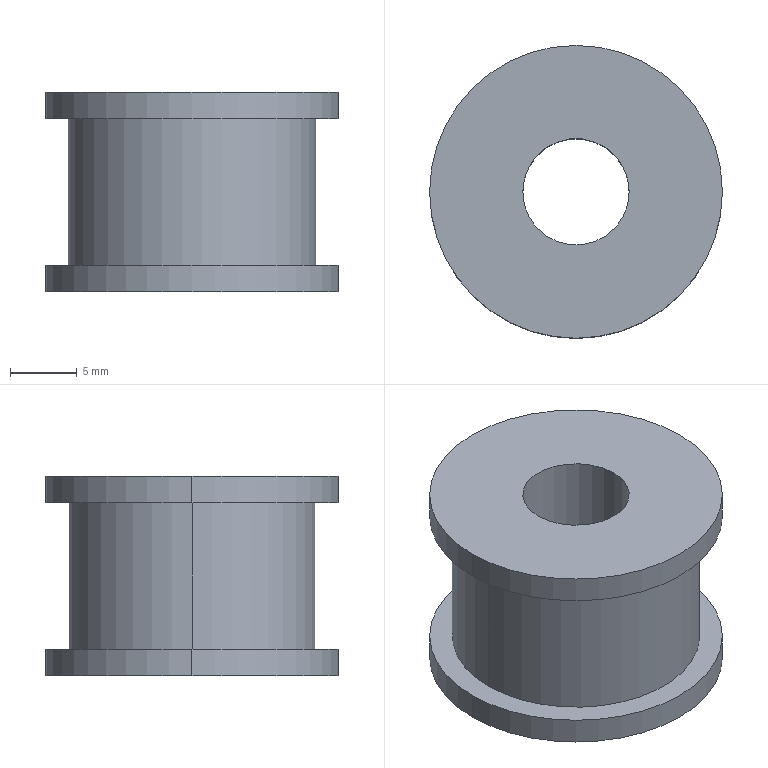Part | SolidWorks | features BaseBody 1 | 1 solid | 12 faces | box 22 x 22 x 15 mm | volume 3752 mm3 | cylinder 8 | plane 4 | commonest cylinder face diameters 22 x4 8 x2 18.59 x2
STEP:
#1=CARTESIAN_POINT('',(-9.295,0.,13.));
#2=VERTEX_POINT('',#1);
#3=CARTESIAN_POINT('',(9.295,0.,13.));
#4=VERTEX_POINT('',#3);
#5=CARTESIAN_POINT('',(0.,0.,13.));
#6=DIRECTION('',(0.,0.,-1.));
#7=DIRECTION('',(-1.,0.,0.));
#8=AXIS2_PLACEMENT_3D('',#5,#6,#7);
#9=CIRCLE('',#8,9.295);
#10=EDGE_CURVE('',#2,#4,#9,.T.);
#11=ORIENTED_EDGE('',*,*,#10,.T.);
#12=CARTESIAN_POINT('',(9.295,0.,2.));
#13=VERTEX_POINT('',#12);
#14=CARTESIAN_POINT('',(9.295,0.,7.5));
#15=DIRECTION('',(0.,0.,-1.));
#16=VECTOR('',#15,1000.);
#17=LINE('',#14,#16);
#18=EDGE_CURVE('',#4,#13,#17,.T.);
#19=ORIENTED_EDGE('',*,*,#18,.T.);
#20=CARTESIAN_POINT('',(-9.295,0.,2.));
#21=VERTEX_POINT('',#20);
#22=CARTESIAN_POINT('',(0.,0.,2.));
#23=DIRECTION('',(0.,0.,1.));
#24=DIRECTION('',(-1.,0.,0.));
#25=AXIS2_PLACEMENT_3D('',#22,#23,#24);
#26=CIRCLE('',#25,9.295);
#27=EDGE_CURVE('',#13,#21,#26,.T.);
#28=ORIENTED_EDGE('',*,*,#27,.T.);
#29=CARTESIAN_POINT('',(-9.295,0.,7.5));
#30=DIRECTION('',(0.,0.,-1.));
#31=VECTOR('',#30,1000.);
#32=LINE('',#29,#31);
#33=EDGE_CURVE('',#2,#21,#32,.T.);
#34=ORIENTED_EDGE('',*,*,#33,.F.);
#35=EDGE_LOOP('',(#11,#19,#28,#34));
#36=FACE_OUTER_BOUND('',#35,.T.);
#37=CARTESIAN_POINT('',(0.,0.,7.5));
#38=DIRECTION('',(0.,0.,-1.));
#39=DIRECTION('',(-1.,0.,0.));
#40=AXIS2_PLACEMENT_3D('',#37,#38,#39);
#41=CYLINDRICAL_SURFACE('',#40,9.295);
#42=ADVANCED_FACE('',(#36),#41,.T.);
#43=CARTESIAN_POINT('',(11.,0.,0.));
#44=VERTEX_POINT('',#43);
#45=CARTESIAN_POINT('',(-11.,0.,0.));
#46=VERTEX_POINT('',#45);
#47=CARTESIAN_POINT('',(0.,0.,0.));
#48=DIRECTION('',(0.,0.,1.));
#49=DIRECTION('',(1.,0.,0.));
#50=AXIS2_PLACEMENT_3D('',#47,#48,#49);
#51=CIRCLE('',#50,11.);
#52=EDGE_CURVE('',#44,#46,#51,.T.);
#53=ORIENTED_EDGE('',*,*,#52,.T.);
#54=CARTESIAN_POINT('',(-11.,0.,2.));
#55=VERTEX_POINT('',#54);
#56=CARTESIAN_POINT('',(-11.,0.,0.));
#57=DIRECTION('',(0.,0.,1.));
#58=VECTOR('',#57,1000.);
#59=LINE('',#56,#58);
#60=EDGE_CURVE('',#46,#55,#59,.T.);
#61=ORIENTED_EDGE('',*,*,#60,.T.);
#62=CARTESIAN_POINT('',(11.,0.,2.));
#63=VERTEX_POINT('',#62);
#64=CARTESIAN_POINT('',(0.,0.,2.));
#65=DIRECTION('',(0.,0.,-1.));
#66=DIRECTION('',(1.,0.,0.));
#67=AXIS2_PLACEMENT_3D('',#64,#65,#66);
#68=CIRCLE('',#67,11.);
#69=EDGE_CURVE('',#55,#63,#68,.T.);
#70=ORIENTED_EDGE('',*,*,#69,.T.);
#71=CARTESIAN_POINT('',(11.,0.,0.));
#72=DIRECTION('',(0.,0.,1.));
#73=VECTOR('',#72,1000.);
#74=LINE('',#71,#73);
#75=EDGE_CURVE('',#44,#63,#74,.T.);
#76=ORIENTED_EDGE('',*,*,#75,.F.);
#77=EDGE_LOOP('',(#53,#61,#70,#76));
#78=FACE_OUTER_BOUND('',#77,.T.);
#79=CARTESIAN_POINT('',(0.,0.,0.));
#80=DIRECTION('',(0.,0.,1.));
#81=DIRECTION('',(1.,0.,0.));
#82=AXIS2_PLACEMENT_3D('',#79,#80,#81);
#83=CYLINDRICAL_SURFACE('',#82,11.);
#84=ADVANCED_FACE('',(#78),#83,.T.);
#85=CARTESIAN_POINT('',(11.,0.,13.));
#86=VERTEX_POINT('',#85);
#87=CARTESIAN_POINT('',(-11.,0.,13.));
#88=VERTEX_POINT('',#87);
#89=CARTESIAN_POINT('',(0.,0.,13.));
#90=DIRECTION('',(0.,0.,1.));
#91=DIRECTION('',(1.,0.,0.));
#92=AXIS2_PLACEMENT_3D('',#89,#90,#91);
#93=CIRCLE('',#92,11.);
#94=EDGE_CURVE('',#86,#88,#93,.T.);
#95=ORIENTED_EDGE('',*,*,#94,.T.);
#96=CARTESIAN_POINT('',(-11.,0.,15.));
#97=VERTEX_POINT('',#96);
#98=CARTESIAN_POINT('',(-11.,0.,0.));
#99=DIRECTION('',(0.,0.,1.));
#100=VECTOR('',#99,1000.);
#101=LINE('',#98,#100);
#102=EDGE_CURVE('',#88,#97,#101,.T.);
#103=ORIENTED_EDGE('',*,*,#102,.T.);
#104=CARTESIAN_POINT('',(11.,0.,15.));
#105=VERTEX_POINT('',#104);
#106=CARTESIAN_POINT('',(0.,0.,15.));
#107=DIRECTION('',(0.,0.,-1.));
#108=DIRECTION('',(1.,0.,0.));
#109=AXIS2_PLACEMENT_3D('',#106,#107,#108);
#110=CIRCLE('',#109,11.);
#111=EDGE_CURVE('',#97,#105,#110,.T.);
#112=ORIENTED_EDGE('',*,*,#111,.T.);
#113=CARTESIAN_POINT('',(11.,0.,0.));
#114=DIRECTION('',(0.,0.,1.));
#115=VECTOR('',#114,1000.);
#116=LINE('',#113,#115);
#117=EDGE_CURVE('',#86,#105,#116,.T.);
#118=ORIENTED_EDGE('',*,*,#117,.F.);
#119=EDGE_LOOP('',(#95,#103,#112,#118));
#120=FACE_OUTER_BOUND('',#119,.T.);
#121=CARTESIAN_POINT('',(0.,0.,0.));
#122=DIRECTION('',(0.,0.,1.));
#123=DIRECTION('',(1.,0.,0.));
#124=AXIS2_PLACEMENT_3D('',#121,#122,#123);
#125=CYLINDRICAL_SURFACE('',#124,11.);
#126=ADVANCED_FACE('',(#120),#125,.T.);
#127=CARTESIAN_POINT('',(-4.,0.,0.));
#128=VERTEX_POINT('',#127);
#129=CARTESIAN_POINT('',(4.,0.,0.));
#130=VERTEX_POINT('',#129);
#131=CARTESIAN_POINT('',(0.,0.,0.));
#132=DIRECTION('',(0.,0.,1.));
#133=DIRECTION('',(1.,0.,0.));
#134=AXIS2_PLACEMENT_3D('',#131,#132,#133);
#135=CIRCLE('',#134,4.);
#136=EDGE_CURVE('',#128,#130,#135,.T.);
#137=ORIENTED_EDGE('',*,*,#136,.F.);
#138=CARTESIAN_POINT('',(-4.,0.,15.));
#139=VERTEX_POINT('',#138);
#140=CARTESIAN_POINT('',(-4.,0.,-19.54));
#141=DIRECTION('',(0.,0.,1.));
#142=VECTOR('',#141,1000.);
#143=LINE('',#140,#142);
#144=EDGE_CURVE('',#128,#139,#143,.T.);
#145=ORIENTED_EDGE('',*,*,#144,.T.);
#146=CARTESIAN_POINT('',(4.,0.,15.));
#147=VERTEX_POINT('',#146);
#148=CARTESIAN_POINT('',(0.,0.,15.));
#149=DIRECTION('',(0.,0.,1.));
#150=DIRECTION('',(1.,0.,0.));
#151=AXIS2_PLACEMENT_3D('',#148,#149,#150);
#152=CIRCLE('',#151,4.);
#153=EDGE_CURVE('',#139,#147,#152,.T.);
#154=ORIENTED_EDGE('',*,*,#153,.T.);
#155=CARTESIAN_POINT('',(4.,0.,-19.54));
#156=DIRECTION('',(0.,0.,1.));
#157=VECTOR('',#156,1000.);
#158=LINE('',#155,#157);
#159=EDGE_CURVE('',#130,#147,#158,.T.);
#160=ORIENTED_EDGE('',*,*,#159,.F.);
#161=EDGE_LOOP('',(#137,#145,#154,#160));
#162=FACE_OUTER_BOUND('',#161,.T.);
#163=CARTESIAN_POINT('',(0.,0.,-19.54));
#164=DIRECTION('',(0.,0.,1.));
#165=DIRECTION('',(1.,0.,0.));
#166=AXIS2_PLACEMENT_3D('',#163,#164,#165);
#167=CYLINDRICAL_SURFACE('',#166,4.);
#168=ADVANCED_FACE('',(#162),#167,.F.);
#169=ORIENTED_EDGE('',*,*,#18,.F.);
#170=CARTESIAN_POINT('',(0.,0.,13.));
#171=DIRECTION('',(0.,0.,-1.));
#172=DIRECTION('',(-1.,0.,0.));
#173=AXIS2_PLACEMENT_3D('',#170,#171,#172);
#174=CIRCLE('',#173,9.295);
#175=EDGE_CURVE('',#4,#2,#174,.T.);
#176=ORIENTED_EDGE('',*,*,#175,.T.);
#177=ORIENTED_EDGE('',*,*,#33,.T.);
#178=CARTESIAN_POINT('',(0.,0.,2.));
#179=DIRECTION('',(0.,0.,1.));
#180=DIRECTION('',(-1.,0.,0.));
#181=AXIS2_PLACEMENT_3D('',#178,#179,#180);
#182=CIRCLE('',#181,9.295);
#183=EDGE_CURVE('',#21,#13,#182,.T.);
#184=ORIENTED_EDGE('',*,*,#183,.T.);
#185=EDGE_LOOP('',(#169,#176,#177,#184));
#186=FACE_OUTER_BOUND('',#185,.T.);
#187=CARTESIAN_POINT('',(0.,0.,7.5));
#188=DIRECTION('',(0.,0.,-1.));
#189=DIRECTION('',(-1.,0.,0.));
#190=AXIS2_PLACEMENT_3D('',#187,#188,#189);
#191=CYLINDRICAL_SURFACE('',#190,9.295);
#192=ADVANCED_FACE('',(#186),#191,.T.);
#193=ORIENTED_EDGE('',*,*,#183,.F.);
#194=ORIENTED_EDGE('',*,*,#27,.F.);
#195=EDGE_LOOP('',(#193,#194));
#196=FACE_BOUND('',#195,.T.);
#197=CARTESIAN_POINT('',(0.,0.,2.));
#198=DIRECTION('',(0.,0.,-1.));
#199=DIRECTION('',(1.,0.,0.));
#200=AXIS2_PLACEMENT_3D('',#197,#198,#199);
#201=CIRCLE('',#200,11.);
#202=EDGE_CURVE('',#63,#55,#201,.T.);
#203=ORIENTED_EDGE('',*,*,#202,.F.);
#204=ORIENTED_EDGE('',*,*,#69,.F.);
#205=EDGE_LOOP('',(#203,#204));
#206=FACE_OUTER_BOUND('',#205,.T.);
#207=CARTESIAN_POINT('',(0.,10.148,2.));
#208=DIRECTION('',(0.,0.,-1.));
#209=DIRECTION('',(-1.,0.,0.));
#210=AXIS2_PLACEMENT_3D('',#207,#208,#209);
#211=PLANE('',#210);
#212=ADVANCED_FACE('',(#196,#206),#211,.F.);
#213=ORIENTED_EDGE('',*,*,#10,.F.);
#214=ORIENTED_EDGE('',*,*,#175,.F.);
#215=EDGE_LOOP('',(#213,#214));
#216=FACE_BOUND('',#215,.T.);
#217=ORIENTED_EDGE('',*,*,#94,.F.);
#218=CARTESIAN_POINT('',(0.,0.,13.));
#219=DIRECTION('',(0.,0.,1.));
#220=DIRECTION('',(1.,0.,0.));
#221=AXIS2_PLACEMENT_3D('',#218,#219,#220);
#222=CIRCLE('',#221,11.);
#223=EDGE_CURVE('',#88,#86,#222,.T.);
#224=ORIENTED_EDGE('',*,*,#223,.F.);
#225=EDGE_LOOP('',(#217,#224));
#226=FACE_OUTER_BOUND('',#225,.T.);
#227=CARTESIAN_POINT('',(0.,10.148,13.));
#228=DIRECTION('',(0.,0.,1.));
#229=DIRECTION('',(1.,0.,0.));
#230=AXIS2_PLACEMENT_3D('',#227,#228,#229);
#231=PLANE('',#230);
#232=ADVANCED_FACE('',(#216,#226),#231,.F.);
#233=ORIENTED_EDGE('',*,*,#60,.F.);
#234=CARTESIAN_POINT('',(0.,0.,0.));
#235=DIRECTION('',(0.,0.,1.));
#236=DIRECTION('',(1.,0.,0.));
#237=AXIS2_PLACEMENT_3D('',#234,#235,#236);
#238=CIRCLE('',#237,11.);
#239=EDGE_CURVE('',#46,#44,#238,.T.);
#240=ORIENTED_EDGE('',*,*,#239,.T.);
#241=ORIENTED_EDGE('',*,*,#75,.T.);
#242=ORIENTED_EDGE('',*,*,#202,.T.);
#243=EDGE_LOOP('',(#233,#240,#241,#242));
#244=FACE_OUTER_BOUND('',#243,.T.);
#245=CARTESIAN_POINT('',(0.,0.,0.));
#246=DIRECTION('',(0.,0.,1.));
#247=DIRECTION('',(1.,0.,0.));
#248=AXIS2_PLACEMENT_3D('',#245,#246,#247);
#249=CYLINDRICAL_SURFACE('',#248,11.);
#250=ADVANCED_FACE('',(#244),#249,.T.);
#251=ORIENTED_EDGE('',*,*,#102,.F.);
#252=ORIENTED_EDGE('',*,*,#223,.T.);
#253=ORIENTED_EDGE('',*,*,#117,.T.);
#254=CARTESIAN_POINT('',(0.,0.,15.));
#255=DIRECTION('',(0.,0.,-1.));
#256=DIRECTION('',(1.,0.,0.));
#257=AXIS2_PLACEMENT_3D('',#254,#255,#256);
#258=CIRCLE('',#257,11.);
#259=EDGE_CURVE('',#105,#97,#258,.T.);
#260=ORIENTED_EDGE('',*,*,#259,.T.);
#261=EDGE_LOOP('',(#251,#252,#253,#260));
#262=FACE_OUTER_BOUND('',#261,.T.);
#263=CARTESIAN_POINT('',(0.,0.,0.));
#264=DIRECTION('',(0.,0.,1.));
#265=DIRECTION('',(1.,0.,0.));
#266=AXIS2_PLACEMENT_3D('',#263,#264,#265);
#267=CYLINDRICAL_SURFACE('',#266,11.);
#268=ADVANCED_FACE('',(#262),#267,.T.);
#269=CARTESIAN_POINT('',(0.,0.,0.));
#270=DIRECTION('',(0.,0.,1.));
#271=DIRECTION('',(1.,0.,0.));
#272=AXIS2_PLACEMENT_3D('',#269,#270,#271);
#273=CIRCLE('',#272,4.);
#274=EDGE_CURVE('',#130,#128,#273,.T.);
#275=ORIENTED_EDGE('',*,*,#274,.T.);
#276=ORIENTED_EDGE('',*,*,#136,.T.);
#277=EDGE_LOOP('',(#275,#276));
#278=FACE_BOUND('',#277,.T.);
#279=ORIENTED_EDGE('',*,*,#52,.F.);
#280=ORIENTED_EDGE('',*,*,#239,.F.);
#281=EDGE_LOOP('',(#279,#280));
#282=FACE_OUTER_BOUND('',#281,.T.);
#283=CARTESIAN_POINT('',(0.,0.,0.));
#284=DIRECTION('',(0.,0.,-1.));
#285=DIRECTION('',(-1.,0.,0.));
#286=AXIS2_PLACEMENT_3D('',#283,#284,#285);
#287=PLANE('',#286);
#288=ADVANCED_FACE('',(#278,#282),#287,.T.);
#289=CARTESIAN_POINT('',(0.,0.,15.));
#290=DIRECTION('',(0.,0.,1.));
#291=DIRECTION('',(1.,0.,0.));
#292=AXIS2_PLACEMENT_3D('',#289,#290,#291);
#293=CIRCLE('',#292,4.);
#294=EDGE_CURVE('',#147,#139,#293,.T.);
#295=ORIENTED_EDGE('',*,*,#294,.F.);
#296=ORIENTED_EDGE('',*,*,#153,.F.);
#297=EDGE_LOOP('',(#295,#296));
#298=FACE_BOUND('',#297,.T.);
#299=ORIENTED_EDGE('',*,*,#259,.F.);
#300=ORIENTED_EDGE('',*,*,#111,.F.);
#301=EDGE_LOOP('',(#299,#300));
#302=FACE_OUTER_BOUND('',#301,.T.);
#303=CARTESIAN_POINT('',(0.,0.,15.));
#304=DIRECTION('',(0.,0.,-1.));
#305=DIRECTION('',(-1.,0.,0.));
#306=AXIS2_PLACEMENT_3D('',#303,#304,#305);
#307=PLANE('',#306);
#308=ADVANCED_FACE('',(#298,#302),#307,.F.);
#309=ORIENTED_EDGE('',*,*,#144,.F.);
#310=ORIENTED_EDGE('',*,*,#274,.F.);
#311=ORIENTED_EDGE('',*,*,#159,.T.);
#312=ORIENTED_EDGE('',*,*,#294,.T.);
#313=EDGE_LOOP('',(#309,#310,#311,#312));
#314=FACE_OUTER_BOUND('',#313,.T.);
#315=CARTESIAN_POINT('',(0.,0.,-19.54));
#316=DIRECTION('',(0.,0.,1.));
#317=DIRECTION('',(1.,0.,0.));
#318=AXIS2_PLACEMENT_3D('',#315,#316,#317);
#319=CYLINDRICAL_SURFACE('',#318,4.);
#320=ADVANCED_FACE('',(#314),#319,.F.);
#321=CLOSED_SHELL('',(#42,#84,#126,#168,#192,#212,#232,#250,#268,#288,#308,#320));
#322=MANIFOLD_SOLID_BREP('',#321);
#323=CARTESIAN_POINT('',(0.,0.,0.));
#324=DIRECTION('',(0.,0.,1.));
#325=DIRECTION('',(1.,0.,0.));
#326=AXIS2_PLACEMENT_3D('',#323,#324,#325);
#327=(LENGTH_UNIT()NAMED_UNIT(*)SI_UNIT(.MILLI.,.METRE.));
#328=UNCERTAINTY_MEASURE_WITH_UNIT(LENGTH_MEASURE(0.00001),#327,'','');
#329=(NAMED_UNIT(*)PLANE_ANGLE_UNIT()SI_UNIT($,.RADIAN.));
#330=(NAMED_UNIT(*)SI_UNIT($,.STERADIAN.)SOLID_ANGLE_UNIT());
#331=(GEOMETRIC_REPRESENTATION_CONTEXT(3)GLOBAL_UNCERTAINTY_ASSIGNED_CONTEXT((#328))GLOBAL_UNIT_ASSIGNED_CONTEXT((#327,#329,#330))REPRESENTATION_CONTEXT('',''));
#332=ADVANCED_BREP_SHAPE_REPRESENTATION('',(#322,#326),#331);